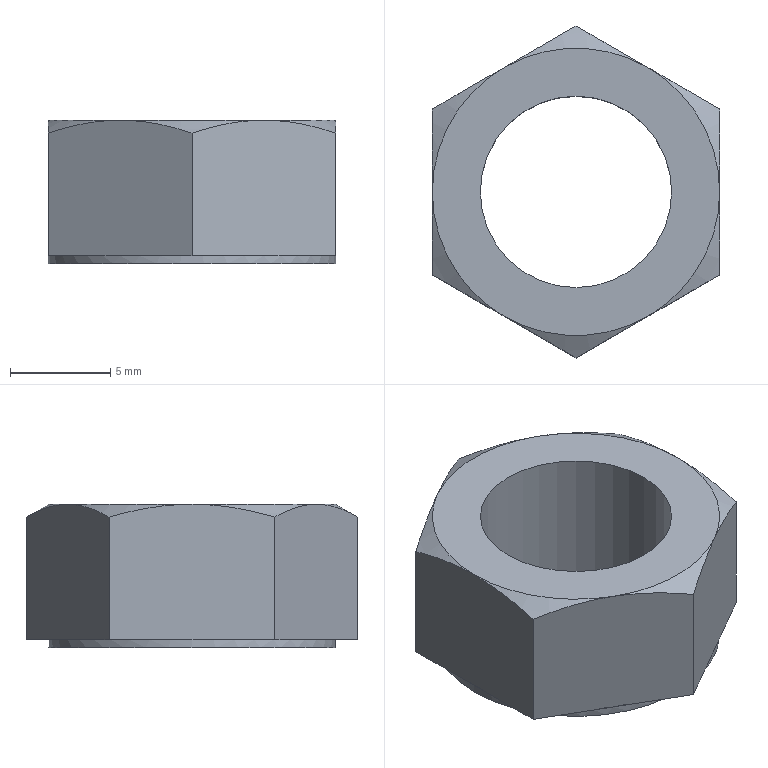Part | NX | features solid 2 | 1 solid | 22 faces | box 14.3 x 16.512 x 7.144 mm | volume 746.181 mm3 | plane 14 | cone 6 | cylinder 2 | commonest cylinder face diameters 9.525 x1 14.3 x1
STEP:
#1=CARTESIAN_POINT('',(3.575,6.192,7.144));
#2=VERTEX_POINT('',#1);
#3=CARTESIAN_POINT('',(0.,8.256,6.505));
#4=VERTEX_POINT('',#3);
#5=CARTESIAN_POINT('',(3.575,6.192,7.144));
#6=CARTESIAN_POINT('',(2.361,6.893,7.144));
#7=CARTESIAN_POINT('',(1.167,7.583,6.894));
#8=CARTESIAN_POINT('',(0.,8.256,6.505));
#9=B_SPLINE_CURVE_WITH_KNOTS('',3,(#5,#6,#7,#8),.UNSPECIFIED.,.F.,.F.,(4,4),(0.004177,0.008339),.UNSPECIFIED.);
#10=EDGE_CURVE('',#2,#4,#9,.T.);
#11=ORIENTED_EDGE('',*,*,#10,.T.);
#12=CARTESIAN_POINT('',(-3.575,6.192,7.144));
#13=VERTEX_POINT('',#12);
#14=CARTESIAN_POINT('',(0.,8.256,6.505));
#15=CARTESIAN_POINT('',(-1.17,7.581,6.895));
#16=CARTESIAN_POINT('',(-2.357,6.895,7.144));
#17=CARTESIAN_POINT('',(-3.575,6.192,7.144));
#18=B_SPLINE_CURVE_WITH_KNOTS('',3,(#14,#15,#16,#17),.UNSPECIFIED.,.F.,.F.,(4,4),(0.000000238,0.004177),.UNSPECIFIED.);
#19=EDGE_CURVE('',#4,#13,#18,.T.);
#20=ORIENTED_EDGE('',*,*,#19,.T.);
#21=CARTESIAN_POINT('',(0.,0.,7.144));
#22=DIRECTION('',(0.,0.,-1.));
#23=DIRECTION('',(-1.,0.,0.));
#24=AXIS2_PLACEMENT_3D('',#21,#22,#23);
#25=CIRCLE('',#24,7.15);
#26=EDGE_CURVE('',#13,#2,#25,.T.);
#27=ORIENTED_EDGE('',*,*,#26,.T.);
#28=EDGE_LOOP('',(#11,#20,#27));
#29=FACE_BOUND('',#28,.T.);
#30=CARTESIAN_POINT('',(0.,0.,7.144));
#31=DIRECTION('',(0.,0.,-1.));
#32=DIRECTION('',(-1.,0.,0.));
#33=AXIS2_PLACEMENT_3D('',#30,#31,#32);
#34=CONICAL_SURFACE('',#33,7.15,1.047);
#35=ADVANCED_FACE('',(#29),#34,.T.);
#36=CARTESIAN_POINT('',(-7.15,0.,7.144));
#37=VERTEX_POINT('',#36);
#38=CARTESIAN_POINT('',(0.,0.,7.144));
#39=DIRECTION('',(0.,0.,-1.));
#40=DIRECTION('',(-1.,0.,0.));
#41=AXIS2_PLACEMENT_3D('',#38,#39,#40);
#42=CIRCLE('',#41,7.15);
#43=EDGE_CURVE('',#37,#13,#42,.T.);
#44=ORIENTED_EDGE('',*,*,#43,.T.);
#45=CARTESIAN_POINT('',(-7.15,4.128,6.505));
#46=VERTEX_POINT('',#45);
#47=CARTESIAN_POINT('',(-3.575,6.192,7.144));
#48=CARTESIAN_POINT('',(-4.789,5.491,7.144));
#49=CARTESIAN_POINT('',(-5.983,4.802,6.894));
#50=CARTESIAN_POINT('',(-7.15,4.128,6.505));
#51=B_SPLINE_CURVE_WITH_KNOTS('',3,(#47,#48,#49,#50),.UNSPECIFIED.,.F.,.F.,(4,4),(0.004177,0.008339),.UNSPECIFIED.);
#52=EDGE_CURVE('',#13,#46,#51,.T.);
#53=ORIENTED_EDGE('',*,*,#52,.T.);
#54=CARTESIAN_POINT('',(-7.15,0.,7.144));
#55=CARTESIAN_POINT('',(-7.15,1.397,7.144));
#56=CARTESIAN_POINT('',(-7.15,2.793,6.891));
#57=CARTESIAN_POINT('',(-7.15,4.128,6.505));
#58=B_SPLINE_CURVE_WITH_KNOTS('',3,(#54,#55,#56,#57),.UNSPECIFIED.,.F.,.F.,(4,4),(0.01176,0.01595),.UNSPECIFIED.);
#59=EDGE_CURVE('',#46,#37,#58,.F.);
#60=ORIENTED_EDGE('',*,*,#59,.T.);
#61=EDGE_LOOP('',(#44,#53,#60));
#62=FACE_BOUND('',#61,.T.);
#63=CARTESIAN_POINT('',(0.,0.,7.144));
#64=DIRECTION('',(0.,0.,-1.));
#65=DIRECTION('',(-1.,0.,0.));
#66=AXIS2_PLACEMENT_3D('',#63,#64,#65);
#67=CONICAL_SURFACE('',#66,7.15,1.047);
#68=ADVANCED_FACE('',(#62),#67,.T.);
#69=CARTESIAN_POINT('',(-3.575,-6.192,7.144));
#70=VERTEX_POINT('',#69);
#71=CARTESIAN_POINT('',(0.,0.,7.144));
#72=DIRECTION('',(0.,0.,-1.));
#73=DIRECTION('',(-1.,0.,0.));
#74=AXIS2_PLACEMENT_3D('',#71,#72,#73);
#75=CIRCLE('',#74,7.15);
#76=EDGE_CURVE('',#70,#37,#75,.T.);
#77=ORIENTED_EDGE('',*,*,#76,.T.);
#78=CARTESIAN_POINT('',(-7.15,-4.128,6.505));
#79=VERTEX_POINT('',#78);
#80=CARTESIAN_POINT('',(-7.15,-4.128,6.505));
#81=CARTESIAN_POINT('',(-7.15,-2.784,6.893));
#82=CARTESIAN_POINT('',(-7.15,-1.396,7.144));
#83=CARTESIAN_POINT('',(-7.15,0.,7.144));
#84=B_SPLINE_CURVE_WITH_KNOTS('',3,(#80,#81,#82,#83),.UNSPECIFIED.,.F.,.F.,(4,4),(0.007586,0.01176),.UNSPECIFIED.);
#85=EDGE_CURVE('',#37,#79,#84,.F.);
#86=ORIENTED_EDGE('',*,*,#85,.T.);
#87=CARTESIAN_POINT('',(-7.15,-4.128,6.505));
#88=CARTESIAN_POINT('',(-5.98,-4.803,6.895));
#89=CARTESIAN_POINT('',(-4.793,-5.489,7.144));
#90=CARTESIAN_POINT('',(-3.575,-6.192,7.144));
#91=B_SPLINE_CURVE_WITH_KNOTS('',3,(#87,#88,#89,#90),.UNSPECIFIED.,.F.,.F.,(4,4),(0.000000238,0.004177),.UNSPECIFIED.);
#92=EDGE_CURVE('',#79,#70,#91,.T.);
#93=ORIENTED_EDGE('',*,*,#92,.T.);
#94=EDGE_LOOP('',(#77,#86,#93));
#95=FACE_BOUND('',#94,.T.);
#96=CARTESIAN_POINT('',(0.,0.,7.144));
#97=DIRECTION('',(0.,0.,-1.));
#98=DIRECTION('',(-1.,0.,0.));
#99=AXIS2_PLACEMENT_3D('',#96,#97,#98);
#100=CONICAL_SURFACE('',#99,7.15,1.047);
#101=ADVANCED_FACE('',(#95),#100,.T.);
#102=CARTESIAN_POINT('',(3.575,-6.192,7.144));
#103=VERTEX_POINT('',#102);
#104=CARTESIAN_POINT('',(0.,0.,7.144));
#105=DIRECTION('',(0.,0.,-1.));
#106=DIRECTION('',(-1.,0.,0.));
#107=AXIS2_PLACEMENT_3D('',#104,#105,#106);
#108=CIRCLE('',#107,7.15);
#109=EDGE_CURVE('',#103,#70,#108,.T.);
#110=ORIENTED_EDGE('',*,*,#109,.T.);
#111=CARTESIAN_POINT('',(0.,-8.256,6.505));
#112=VERTEX_POINT('',#111);
#113=CARTESIAN_POINT('',(-3.575,-6.192,7.144));
#114=CARTESIAN_POINT('',(-2.361,-6.893,7.144));
#115=CARTESIAN_POINT('',(-1.167,-7.583,6.894));
#116=CARTESIAN_POINT('',(0.,-8.256,6.505));
#117=B_SPLINE_CURVE_WITH_KNOTS('',3,(#113,#114,#115,#116),.UNSPECIFIED.,.F.,.F.,(4,4),(0.004177,0.008339),.UNSPECIFIED.);
#118=EDGE_CURVE('',#70,#112,#117,.T.);
#119=ORIENTED_EDGE('',*,*,#118,.T.);
#120=CARTESIAN_POINT('',(0.,-8.256,6.505));
#121=CARTESIAN_POINT('',(1.17,-7.581,6.895));
#122=CARTESIAN_POINT('',(2.357,-6.895,7.144));
#123=CARTESIAN_POINT('',(3.575,-6.192,7.144));
#124=B_SPLINE_CURVE_WITH_KNOTS('',3,(#120,#121,#122,#123),.UNSPECIFIED.,.F.,.F.,(4,4),(0.000000238,0.004177),.UNSPECIFIED.);
#125=EDGE_CURVE('',#112,#103,#124,.T.);
#126=ORIENTED_EDGE('',*,*,#125,.T.);
#127=EDGE_LOOP('',(#110,#119,#126));
#128=FACE_BOUND('',#127,.T.);
#129=CARTESIAN_POINT('',(0.,0.,7.144));
#130=DIRECTION('',(0.,0.,-1.));
#131=DIRECTION('',(-1.,0.,0.));
#132=AXIS2_PLACEMENT_3D('',#129,#130,#131);
#133=CONICAL_SURFACE('',#132,7.15,1.047);
#134=ADVANCED_FACE('',(#128),#133,.T.);
#135=CARTESIAN_POINT('',(7.15,0.,7.144));
#136=VERTEX_POINT('',#135);
#137=CARTESIAN_POINT('',(0.,0.,7.144));
#138=DIRECTION('',(0.,0.,-1.));
#139=DIRECTION('',(-1.,0.,0.));
#140=AXIS2_PLACEMENT_3D('',#137,#138,#139);
#141=CIRCLE('',#140,7.15);
#142=EDGE_CURVE('',#136,#103,#141,.T.);
#143=ORIENTED_EDGE('',*,*,#142,.T.);
#144=CARTESIAN_POINT('',(7.15,-4.128,6.505));
#145=VERTEX_POINT('',#144);
#146=CARTESIAN_POINT('',(3.575,-6.192,7.144));
#147=CARTESIAN_POINT('',(4.789,-5.491,7.144));
#148=CARTESIAN_POINT('',(5.983,-4.802,6.894));
#149=CARTESIAN_POINT('',(7.15,-4.128,6.505));
#150=B_SPLINE_CURVE_WITH_KNOTS('',3,(#146,#147,#148,#149),.UNSPECIFIED.,.F.,.F.,(4,4),(0.004177,0.008339),.UNSPECIFIED.);
#151=EDGE_CURVE('',#103,#145,#150,.T.);
#152=ORIENTED_EDGE('',*,*,#151,.T.);
#153=CARTESIAN_POINT('',(7.15,-4.128,6.505));
#154=CARTESIAN_POINT('',(7.15,-2.784,6.893));
#155=CARTESIAN_POINT('',(7.15,-1.396,7.144));
#156=CARTESIAN_POINT('',(7.15,0.,7.144));
#157=B_SPLINE_CURVE_WITH_KNOTS('',3,(#153,#154,#155,#156),.UNSPECIFIED.,.F.,.F.,(4,4),(0.007586,0.01176),.UNSPECIFIED.);
#158=EDGE_CURVE('',#145,#136,#157,.T.);
#159=ORIENTED_EDGE('',*,*,#158,.T.);
#160=EDGE_LOOP('',(#143,#152,#159));
#161=FACE_BOUND('',#160,.T.);
#162=CARTESIAN_POINT('',(0.,0.,7.144));
#163=DIRECTION('',(0.,0.,-1.));
#164=DIRECTION('',(-1.,0.,0.));
#165=AXIS2_PLACEMENT_3D('',#162,#163,#164);
#166=CONICAL_SURFACE('',#165,7.15,1.047);
#167=ADVANCED_FACE('',(#161),#166,.T.);
#168=CARTESIAN_POINT('',(0.,0.,7.144));
#169=DIRECTION('',(0.,0.,-1.));
#170=DIRECTION('',(-1.,0.,0.));
#171=AXIS2_PLACEMENT_3D('',#168,#169,#170);
#172=CIRCLE('',#171,7.15);
#173=EDGE_CURVE('',#2,#136,#172,.T.);
#174=ORIENTED_EDGE('',*,*,#173,.T.);
#175=CARTESIAN_POINT('',(7.15,4.128,6.505));
#176=VERTEX_POINT('',#175);
#177=CARTESIAN_POINT('',(7.15,0.,7.144));
#178=CARTESIAN_POINT('',(7.15,1.397,7.144));
#179=CARTESIAN_POINT('',(7.15,2.793,6.891));
#180=CARTESIAN_POINT('',(7.15,4.128,6.505));
#181=B_SPLINE_CURVE_WITH_KNOTS('',3,(#177,#178,#179,#180),.UNSPECIFIED.,.F.,.F.,(4,4),(0.01176,0.01595),.UNSPECIFIED.);
#182=EDGE_CURVE('',#136,#176,#181,.T.);
#183=ORIENTED_EDGE('',*,*,#182,.T.);
#184=CARTESIAN_POINT('',(7.15,4.128,6.505));
#185=CARTESIAN_POINT('',(5.98,4.803,6.895));
#186=CARTESIAN_POINT('',(4.793,5.489,7.144));
#187=CARTESIAN_POINT('',(3.575,6.192,7.144));
#188=B_SPLINE_CURVE_WITH_KNOTS('',3,(#184,#185,#186,#187),.UNSPECIFIED.,.F.,.F.,(4,4),(0.000000238,0.004177),.UNSPECIFIED.);
#189=EDGE_CURVE('',#176,#2,#188,.T.);
#190=ORIENTED_EDGE('',*,*,#189,.T.);
#191=EDGE_LOOP('',(#174,#183,#190));
#192=FACE_BOUND('',#191,.T.);
#193=CARTESIAN_POINT('',(0.,0.,7.144));
#194=DIRECTION('',(0.,0.,-1.));
#195=DIRECTION('',(-1.,0.,0.));
#196=AXIS2_PLACEMENT_3D('',#193,#194,#195);
#197=CONICAL_SURFACE('',#196,7.15,1.047);
#198=ADVANCED_FACE('',(#192),#197,.T.);
#199=CARTESIAN_POINT('',(3.575,-6.192,0.4064));
#200=VERTEX_POINT('',#199);
#201=CARTESIAN_POINT('',(0.,-8.256,0.4064));
#202=VERTEX_POINT('',#201);
#203=CARTESIAN_POINT('',(11.619,-1.548,0.4064));
#204=DIRECTION('',(-0.866,-0.5,0.));
#205=VECTOR('',#204,1000.);
#206=LINE('',#203,#205);
#207=EDGE_CURVE('',#200,#202,#206,.T.);
#208=ORIENTED_EDGE('',*,*,#207,.T.);
#209=CARTESIAN_POINT('',(-3.575,-6.192,0.4064));
#210=VERTEX_POINT('',#209);
#211=CARTESIAN_POINT('',(4.469,-10.836,0.4064));
#212=DIRECTION('',(-0.866,0.5,0.));
#213=VECTOR('',#212,1000.);
#214=LINE('',#211,#213);
#215=EDGE_CURVE('',#202,#210,#214,.T.);
#216=ORIENTED_EDGE('',*,*,#215,.T.);
#217=CARTESIAN_POINT('',(0.,0.,0.4064));
#218=DIRECTION('',(0.,0.,-1.));
#219=DIRECTION('',(-1.,0.,0.));
#220=AXIS2_PLACEMENT_3D('',#217,#218,#219);
#221=CIRCLE('',#220,7.15);
#222=EDGE_CURVE('',#200,#210,#221,.T.);
#223=ORIENTED_EDGE('',*,*,#222,.F.);
#224=EDGE_LOOP('',(#208,#216,#223));
#225=FACE_BOUND('',#224,.T.);
#226=CARTESIAN_POINT('',(10.725,0.,0.4064));
#227=DIRECTION('',(0.,0.,1.));
#228=DIRECTION('',(1.,0.,0.));
#229=AXIS2_PLACEMENT_3D('',#226,#227,#228);
#230=PLANE('',#229);
#231=ADVANCED_FACE('',(#225),#230,.F.);
#232=CARTESIAN_POINT('',(-7.15,0.,0.4064));
#233=VERTEX_POINT('',#232);
#234=CARTESIAN_POINT('',(0.,0.,0.4064));
#235=DIRECTION('',(0.,0.,-1.));
#236=DIRECTION('',(-1.,0.,0.));
#237=AXIS2_PLACEMENT_3D('',#234,#235,#236);
#238=CIRCLE('',#237,7.15);
#239=EDGE_CURVE('',#210,#233,#238,.T.);
#240=ORIENTED_EDGE('',*,*,#239,.F.);
#241=CARTESIAN_POINT('',(-7.15,-4.128,0.4064));
#242=VERTEX_POINT('',#241);
#243=CARTESIAN_POINT('',(4.469,-10.836,0.4064));
#244=DIRECTION('',(-0.866,0.5,0.));
#245=VECTOR('',#244,1000.);
#246=LINE('',#243,#245);
#247=EDGE_CURVE('',#210,#242,#246,.T.);
#248=ORIENTED_EDGE('',*,*,#247,.T.);
#249=CARTESIAN_POINT('',(-7.15,0.,0.4064));
#250=DIRECTION('',(0.,1.,0.));
#251=VECTOR('',#250,1000.);
#252=LINE('',#249,#251);
#253=EDGE_CURVE('',#242,#233,#252,.T.);
#254=ORIENTED_EDGE('',*,*,#253,.T.);
#255=EDGE_LOOP('',(#240,#248,#254));
#256=FACE_BOUND('',#255,.T.);
#257=CARTESIAN_POINT('',(10.725,0.,0.4064));
#258=DIRECTION('',(0.,0.,1.));
#259=DIRECTION('',(1.,0.,0.));
#260=AXIS2_PLACEMENT_3D('',#257,#258,#259);
#261=PLANE('',#260);
#262=ADVANCED_FACE('',(#256),#261,.F.);
#263=CARTESIAN_POINT('',(-3.575,6.192,0.4064));
#264=VERTEX_POINT('',#263);
#265=CARTESIAN_POINT('',(0.,0.,0.4064));
#266=DIRECTION('',(0.,0.,-1.));
#267=DIRECTION('',(-1.,0.,0.));
#268=AXIS2_PLACEMENT_3D('',#265,#266,#267);
#269=CIRCLE('',#268,7.15);
#270=EDGE_CURVE('',#233,#264,#269,.T.);
#271=ORIENTED_EDGE('',*,*,#270,.F.);
#272=CARTESIAN_POINT('',(-7.15,4.128,0.4064));
#273=VERTEX_POINT('',#272);
#274=CARTESIAN_POINT('',(-7.15,0.,0.4064));
#275=DIRECTION('',(0.,1.,0.));
#276=VECTOR('',#275,1000.);
#277=LINE('',#274,#276);
#278=EDGE_CURVE('',#233,#273,#277,.T.);
#279=ORIENTED_EDGE('',*,*,#278,.T.);
#280=CARTESIAN_POINT('',(4.469,10.836,0.4064));
#281=DIRECTION('',(0.866,0.5,0.));
#282=VECTOR('',#281,1000.);
#283=LINE('',#280,#282);
#284=EDGE_CURVE('',#273,#264,#283,.T.);
#285=ORIENTED_EDGE('',*,*,#284,.T.);
#286=EDGE_LOOP('',(#271,#279,#285));
#287=FACE_BOUND('',#286,.T.);
#288=CARTESIAN_POINT('',(10.725,0.,0.4064));
#289=DIRECTION('',(0.,0.,1.));
#290=DIRECTION('',(1.,0.,0.));
#291=AXIS2_PLACEMENT_3D('',#288,#289,#290);
#292=PLANE('',#291);
#293=ADVANCED_FACE('',(#287),#292,.F.);
#294=CARTESIAN_POINT('',(7.15,0.,0.4064));
#295=VERTEX_POINT('',#294);
#296=CARTESIAN_POINT('',(7.15,-4.128,0.4064));
#297=VERTEX_POINT('',#296);
#298=CARTESIAN_POINT('',(7.15,0.,0.4064));
#299=DIRECTION('',(0.,-1.,0.));
#300=VECTOR('',#299,1000.);
#301=LINE('',#298,#300);
#302=EDGE_CURVE('',#295,#297,#301,.T.);
#303=ORIENTED_EDGE('',*,*,#302,.T.);
#304=CARTESIAN_POINT('',(11.619,-1.548,0.4064));
#305=DIRECTION('',(-0.866,-0.5,0.));
#306=VECTOR('',#305,1000.);
#307=LINE('',#304,#306);
#308=EDGE_CURVE('',#297,#200,#307,.T.);
#309=ORIENTED_EDGE('',*,*,#308,.T.);
#310=CARTESIAN_POINT('',(0.,0.,0.4064));
#311=DIRECTION('',(0.,0.,-1.));
#312=DIRECTION('',(-1.,0.,0.));
#313=AXIS2_PLACEMENT_3D('',#310,#311,#312);
#314=CIRCLE('',#313,7.15);
#315=EDGE_CURVE('',#295,#200,#314,.T.);
#316=ORIENTED_EDGE('',*,*,#315,.F.);
#317=EDGE_LOOP('',(#303,#309,#316));
#318=FACE_BOUND('',#317,.T.);
#319=CARTESIAN_POINT('',(10.725,0.,0.4064));
#320=DIRECTION('',(0.,0.,1.));
#321=DIRECTION('',(1.,0.,0.));
#322=AXIS2_PLACEMENT_3D('',#319,#320,#321);
#323=PLANE('',#322);
#324=ADVANCED_FACE('',(#318),#323,.F.);
#325=CARTESIAN_POINT('',(3.575,6.192,0.4064));
#326=VERTEX_POINT('',#325);
#327=CARTESIAN_POINT('',(0.,0.,0.4064));
#328=DIRECTION('',(0.,0.,-1.));
#329=DIRECTION('',(-1.,0.,0.));
#330=AXIS2_PLACEMENT_3D('',#327,#328,#329);
#331=CIRCLE('',#330,7.15);
#332=EDGE_CURVE('',#264,#326,#331,.T.);
#333=ORIENTED_EDGE('',*,*,#332,.F.);
#334=CARTESIAN_POINT('',(0.,8.256,0.4064));
#335=VERTEX_POINT('',#334);
#336=CARTESIAN_POINT('',(4.469,10.836,0.4064));
#337=DIRECTION('',(0.866,0.5,0.));
#338=VECTOR('',#337,1000.);
#339=LINE('',#336,#338);
#340=EDGE_CURVE('',#264,#335,#339,.T.);
#341=ORIENTED_EDGE('',*,*,#340,.T.);
#342=CARTESIAN_POINT('',(11.619,1.548,0.4064));
#343=DIRECTION('',(0.866,-0.5,0.));
#344=VECTOR('',#343,1000.);
#345=LINE('',#342,#344);
#346=EDGE_CURVE('',#335,#326,#345,.T.);
#347=ORIENTED_EDGE('',*,*,#346,.T.);
#348=EDGE_LOOP('',(#333,#341,#347));
#349=FACE_BOUND('',#348,.T.);
#350=CARTESIAN_POINT('',(10.725,0.,0.4064));
#351=DIRECTION('',(0.,0.,1.));
#352=DIRECTION('',(1.,0.,0.));
#353=AXIS2_PLACEMENT_3D('',#350,#351,#352);
#354=PLANE('',#353);
#355=ADVANCED_FACE('',(#349),#354,.F.);
#356=CARTESIAN_POINT('',(7.15,4.128,0.4064));
#357=VERTEX_POINT('',#356);
#358=CARTESIAN_POINT('',(11.619,1.548,0.4064));
#359=DIRECTION('',(0.866,-0.5,0.));
#360=VECTOR('',#359,1000.);
#361=LINE('',#358,#360);
#362=EDGE_CURVE('',#326,#357,#361,.T.);
#363=ORIENTED_EDGE('',*,*,#362,.T.);
#364=CARTESIAN_POINT('',(7.15,0.,0.4064));
#365=DIRECTION('',(0.,-1.,0.));
#366=VECTOR('',#365,1000.);
#367=LINE('',#364,#366);
#368=EDGE_CURVE('',#357,#295,#367,.T.);
#369=ORIENTED_EDGE('',*,*,#368,.T.);
#370=CARTESIAN_POINT('',(0.,0.,0.4064));
#371=DIRECTION('',(0.,0.,-1.));
#372=DIRECTION('',(-1.,0.,0.));
#373=AXIS2_PLACEMENT_3D('',#370,#371,#372);
#374=CIRCLE('',#373,7.15);
#375=EDGE_CURVE('',#326,#295,#374,.T.);
#376=ORIENTED_EDGE('',*,*,#375,.F.);
#377=EDGE_LOOP('',(#363,#369,#376));
#378=FACE_BOUND('',#377,.T.);
#379=CARTESIAN_POINT('',(10.725,0.,0.4064));
#380=DIRECTION('',(0.,0.,1.));
#381=DIRECTION('',(1.,0.,0.));
#382=AXIS2_PLACEMENT_3D('',#379,#380,#381);
#383=PLANE('',#382);
#384=ADVANCED_FACE('',(#378),#383,.F.);
#385=ORIENTED_EDGE('',*,*,#43,.F.);
#386=ORIENTED_EDGE('',*,*,#76,.F.);
#387=ORIENTED_EDGE('',*,*,#109,.F.);
#388=ORIENTED_EDGE('',*,*,#142,.F.);
#389=ORIENTED_EDGE('',*,*,#173,.F.);
#390=ORIENTED_EDGE('',*,*,#26,.F.);
#391=EDGE_LOOP('',(#385,#386,#387,#388,#389,#390));
#392=FACE_BOUND('',#391,.T.);
#393=CARTESIAN_POINT('',(-4.763,0.,7.144));
#394=VERTEX_POINT('',#393);
#395=CARTESIAN_POINT('',(0.,0.,7.144));
#396=DIRECTION('',(0.,0.,-1.));
#397=DIRECTION('',(-1.,0.,0.));
#398=AXIS2_PLACEMENT_3D('',#395,#396,#397);
#399=CIRCLE('',#398,4.763);
#400=EDGE_CURVE('',#394,#394,#399,.T.);
#401=ORIENTED_EDGE('',*,*,#400,.T.);
#402=EDGE_LOOP('',(#401));
#403=FACE_BOUND('',#402,.T.);
#404=CARTESIAN_POINT('',(4.763,0.,7.144));
#405=DIRECTION('',(0.,0.,-1.));
#406=DIRECTION('',(-1.,0.,0.));
#407=AXIS2_PLACEMENT_3D('',#404,#405,#406);
#408=PLANE('',#407);
#409=ADVANCED_FACE('',(#392,#403),#408,.F.);
#410=CARTESIAN_POINT('',(-7.15,0.,0.));
#411=VERTEX_POINT('',#410);
#412=CARTESIAN_POINT('',(0.,0.,0.));
#413=DIRECTION('',(0.,0.,-1.));
#414=DIRECTION('',(-1.,0.,0.));
#415=AXIS2_PLACEMENT_3D('',#412,#413,#414);
#416=CIRCLE('',#415,7.15);
#417=EDGE_CURVE('',#411,#411,#416,.T.);
#418=ORIENTED_EDGE('',*,*,#417,.F.);
#419=EDGE_LOOP('',(#418));
#420=FACE_BOUND('',#419,.T.);
#421=ORIENTED_EDGE('',*,*,#270,.T.);
#422=ORIENTED_EDGE('',*,*,#332,.T.);
#423=ORIENTED_EDGE('',*,*,#375,.T.);
#424=ORIENTED_EDGE('',*,*,#315,.T.);
#425=ORIENTED_EDGE('',*,*,#222,.T.);
#426=ORIENTED_EDGE('',*,*,#239,.T.);
#427=EDGE_LOOP('',(#421,#422,#423,#424,#425,#426));
#428=FACE_BOUND('',#427,.T.);
#429=CARTESIAN_POINT('',(0.,0.,0.));
#430=DIRECTION('',(0.,0.,-1.));
#431=DIRECTION('',(-1.,0.,0.));
#432=AXIS2_PLACEMENT_3D('',#429,#430,#431);
#433=CYLINDRICAL_SURFACE('',#432,7.15);
#434=ADVANCED_FACE('',(#420,#428),#433,.T.);
#435=CARTESIAN_POINT('',(-4.763,0.,0.));
#436=VERTEX_POINT('',#435);
#437=CARTESIAN_POINT('',(0.,0.,0.));
#438=DIRECTION('',(0.,0.,-1.));
#439=DIRECTION('',(-1.,0.,0.));
#440=AXIS2_PLACEMENT_3D('',#437,#438,#439);
#441=CIRCLE('',#440,4.763);
#442=EDGE_CURVE('',#436,#436,#441,.T.);
#443=ORIENTED_EDGE('',*,*,#442,.F.);
#444=EDGE_LOOP('',(#443));
#445=FACE_BOUND('',#444,.T.);
#446=ORIENTED_EDGE('',*,*,#417,.T.);
#447=EDGE_LOOP('',(#446));
#448=FACE_BOUND('',#447,.T.);
#449=CARTESIAN_POINT('',(7.15,0.,0.));
#450=DIRECTION('',(0.,0.,1.));
#451=DIRECTION('',(1.,0.,0.));
#452=AXIS2_PLACEMENT_3D('',#449,#450,#451);
#453=PLANE('',#452);
#454=ADVANCED_FACE('',(#445,#448),#453,.F.);
#455=ORIENTED_EDGE('',*,*,#400,.F.);
#456=EDGE_LOOP('',(#455));
#457=FACE_BOUND('',#456,.T.);
#458=ORIENTED_EDGE('',*,*,#442,.T.);
#459=EDGE_LOOP('',(#458));
#460=FACE_BOUND('',#459,.T.);
#461=CARTESIAN_POINT('',(0.,0.,0.));
#462=DIRECTION('',(0.,0.,-1.));
#463=DIRECTION('',(-1.,0.,0.));
#464=AXIS2_PLACEMENT_3D('',#461,#462,#463);
#465=CYLINDRICAL_SURFACE('',#464,4.763);
#466=ADVANCED_FACE('',(#457,#460),#465,.F.);
#467=ORIENTED_EDGE('',*,*,#19,.F.);
#468=CARTESIAN_POINT('',(0.,8.256,7.858));
#469=DIRECTION('',(0.,0.,-1.));
#470=VECTOR('',#469,1000.);
#471=LINE('',#468,#470);
#472=EDGE_CURVE('',#4,#335,#471,.T.);
#473=ORIENTED_EDGE('',*,*,#472,.T.);
#474=ORIENTED_EDGE('',*,*,#340,.F.);
#475=ORIENTED_EDGE('',*,*,#284,.F.);
#476=CARTESIAN_POINT('',(-7.15,4.128,7.858));
#477=DIRECTION('',(0.,0.,-1.));
#478=VECTOR('',#477,1000.);
#479=LINE('',#476,#478);
#480=EDGE_CURVE('',#46,#273,#479,.T.);
#481=ORIENTED_EDGE('',*,*,#480,.F.);
#482=ORIENTED_EDGE('',*,*,#52,.F.);
#483=EDGE_LOOP('',(#467,#473,#474,#475,#481,#482));
#484=FACE_BOUND('',#483,.T.);
#485=CARTESIAN_POINT('',(0.,8.256,7.858));
#486=DIRECTION('',(0.5,-0.866,0.));
#487=DIRECTION('',(0.866,0.5,0.));
#488=AXIS2_PLACEMENT_3D('',#485,#486,#487);
#489=PLANE('',#488);
#490=ADVANCED_FACE('',(#484),#489,.F.);
#491=ORIENTED_EDGE('',*,*,#59,.F.);
#492=ORIENTED_EDGE('',*,*,#480,.T.);
#493=ORIENTED_EDGE('',*,*,#278,.F.);
#494=ORIENTED_EDGE('',*,*,#253,.F.);
#495=CARTESIAN_POINT('',(-7.15,-4.128,7.858));
#496=DIRECTION('',(0.,0.,-1.));
#497=VECTOR('',#496,1000.);
#498=LINE('',#495,#497);
#499=EDGE_CURVE('',#79,#242,#498,.T.);
#500=ORIENTED_EDGE('',*,*,#499,.F.);
#501=ORIENTED_EDGE('',*,*,#85,.F.);
#502=EDGE_LOOP('',(#491,#492,#493,#494,#500,#501));
#503=FACE_BOUND('',#502,.T.);
#504=CARTESIAN_POINT('',(-7.15,4.128,7.858));
#505=DIRECTION('',(1.,0.,0.));
#506=DIRECTION('',(0.,1.,0.));
#507=AXIS2_PLACEMENT_3D('',#504,#505,#506);
#508=PLANE('',#507);
#509=ADVANCED_FACE('',(#503),#508,.F.);
#510=ORIENTED_EDGE('',*,*,#92,.F.);
#511=ORIENTED_EDGE('',*,*,#499,.T.);
#512=ORIENTED_EDGE('',*,*,#247,.F.);
#513=ORIENTED_EDGE('',*,*,#215,.F.);
#514=CARTESIAN_POINT('',(0.,-8.256,7.858));
#515=DIRECTION('',(0.,0.,-1.));
#516=VECTOR('',#515,1000.);
#517=LINE('',#514,#516);
#518=EDGE_CURVE('',#112,#202,#517,.T.);
#519=ORIENTED_EDGE('',*,*,#518,.F.);
#520=ORIENTED_EDGE('',*,*,#118,.F.);
#521=EDGE_LOOP('',(#510,#511,#512,#513,#519,#520));
#522=FACE_BOUND('',#521,.T.);
#523=CARTESIAN_POINT('',(-7.15,-4.128,7.858));
#524=DIRECTION('',(0.5,0.866,0.));
#525=DIRECTION('',(-0.866,0.5,0.));
#526=AXIS2_PLACEMENT_3D('',#523,#524,#525);
#527=PLANE('',#526);
#528=ADVANCED_FACE('',(#522),#527,.F.);
#529=ORIENTED_EDGE('',*,*,#125,.F.);
#530=ORIENTED_EDGE('',*,*,#518,.T.);
#531=ORIENTED_EDGE('',*,*,#207,.F.);
#532=ORIENTED_EDGE('',*,*,#308,.F.);
#533=CARTESIAN_POINT('',(7.15,-4.128,7.858));
#534=DIRECTION('',(0.,0.,-1.));
#535=VECTOR('',#534,1000.);
#536=LINE('',#533,#535);
#537=EDGE_CURVE('',#145,#297,#536,.T.);
#538=ORIENTED_EDGE('',*,*,#537,.F.);
#539=ORIENTED_EDGE('',*,*,#151,.F.);
#540=EDGE_LOOP('',(#529,#530,#531,#532,#538,#539));
#541=FACE_BOUND('',#540,.T.);
#542=CARTESIAN_POINT('',(0.,-8.256,7.858));
#543=DIRECTION('',(-0.5,0.866,0.));
#544=DIRECTION('',(-0.866,-0.5,0.));
#545=AXIS2_PLACEMENT_3D('',#542,#543,#544);
#546=PLANE('',#545);
#547=ADVANCED_FACE('',(#541),#546,.F.);
#548=ORIENTED_EDGE('',*,*,#158,.F.);
#549=ORIENTED_EDGE('',*,*,#537,.T.);
#550=ORIENTED_EDGE('',*,*,#302,.F.);
#551=ORIENTED_EDGE('',*,*,#368,.F.);
#552=CARTESIAN_POINT('',(7.15,4.128,7.858));
#553=DIRECTION('',(0.,0.,-1.));
#554=VECTOR('',#553,1000.);
#555=LINE('',#552,#554);
#556=EDGE_CURVE('',#176,#357,#555,.T.);
#557=ORIENTED_EDGE('',*,*,#556,.F.);
#558=ORIENTED_EDGE('',*,*,#182,.F.);
#559=EDGE_LOOP('',(#548,#549,#550,#551,#557,#558));
#560=FACE_BOUND('',#559,.T.);
#561=CARTESIAN_POINT('',(7.15,-4.128,7.858));
#562=DIRECTION('',(-1.,0.,0.));
#563=DIRECTION('',(0.,0.,1.));
#564=AXIS2_PLACEMENT_3D('',#561,#562,#563);
#565=PLANE('',#564);
#566=ADVANCED_FACE('',(#560),#565,.F.);
#567=ORIENTED_EDGE('',*,*,#189,.F.);
#568=ORIENTED_EDGE('',*,*,#556,.T.);
#569=ORIENTED_EDGE('',*,*,#362,.F.);
#570=ORIENTED_EDGE('',*,*,#346,.F.);
#571=ORIENTED_EDGE('',*,*,#472,.F.);
#572=ORIENTED_EDGE('',*,*,#10,.F.);
#573=EDGE_LOOP('',(#567,#568,#569,#570,#571,#572));
#574=FACE_BOUND('',#573,.T.);
#575=CARTESIAN_POINT('',(7.15,4.128,7.858));
#576=DIRECTION('',(-0.5,-0.866,0.));
#577=DIRECTION('',(0.866,-0.5,0.));
#578=AXIS2_PLACEMENT_3D('',#575,#576,#577);
#579=PLANE('',#578);
#580=ADVANCED_FACE('',(#574),#579,.F.);
#581=CLOSED_SHELL('',(#35,#68,#101,#134,#167,#198,#231,#262,#293,#324,#355,#384,#409,#434,#454,#466,#490,#509,#528,#547,#566,#580));
#582=MANIFOLD_SOLID_BREP('',#581);
#583=(LENGTH_UNIT()NAMED_UNIT(*)SI_UNIT(.MILLI.,.METRE.));
#584=UNCERTAINTY_MEASURE_WITH_UNIT(LENGTH_MEASURE(0.0508),#583,'','');
#585=(NAMED_UNIT(*)PLANE_ANGLE_UNIT()SI_UNIT($,.RADIAN.));
#586=(NAMED_UNIT(*)SI_UNIT($,.STERADIAN.)SOLID_ANGLE_UNIT());
#587=(GEOMETRIC_REPRESENTATION_CONTEXT(3)GLOBAL_UNCERTAINTY_ASSIGNED_CONTEXT((#584))GLOBAL_UNIT_ASSIGNED_CONTEXT((#583,#585,#586))REPRESENTATION_CONTEXT('',''));
#588=ADVANCED_BREP_SHAPE_REPRESENTATION('',(#582),#587);